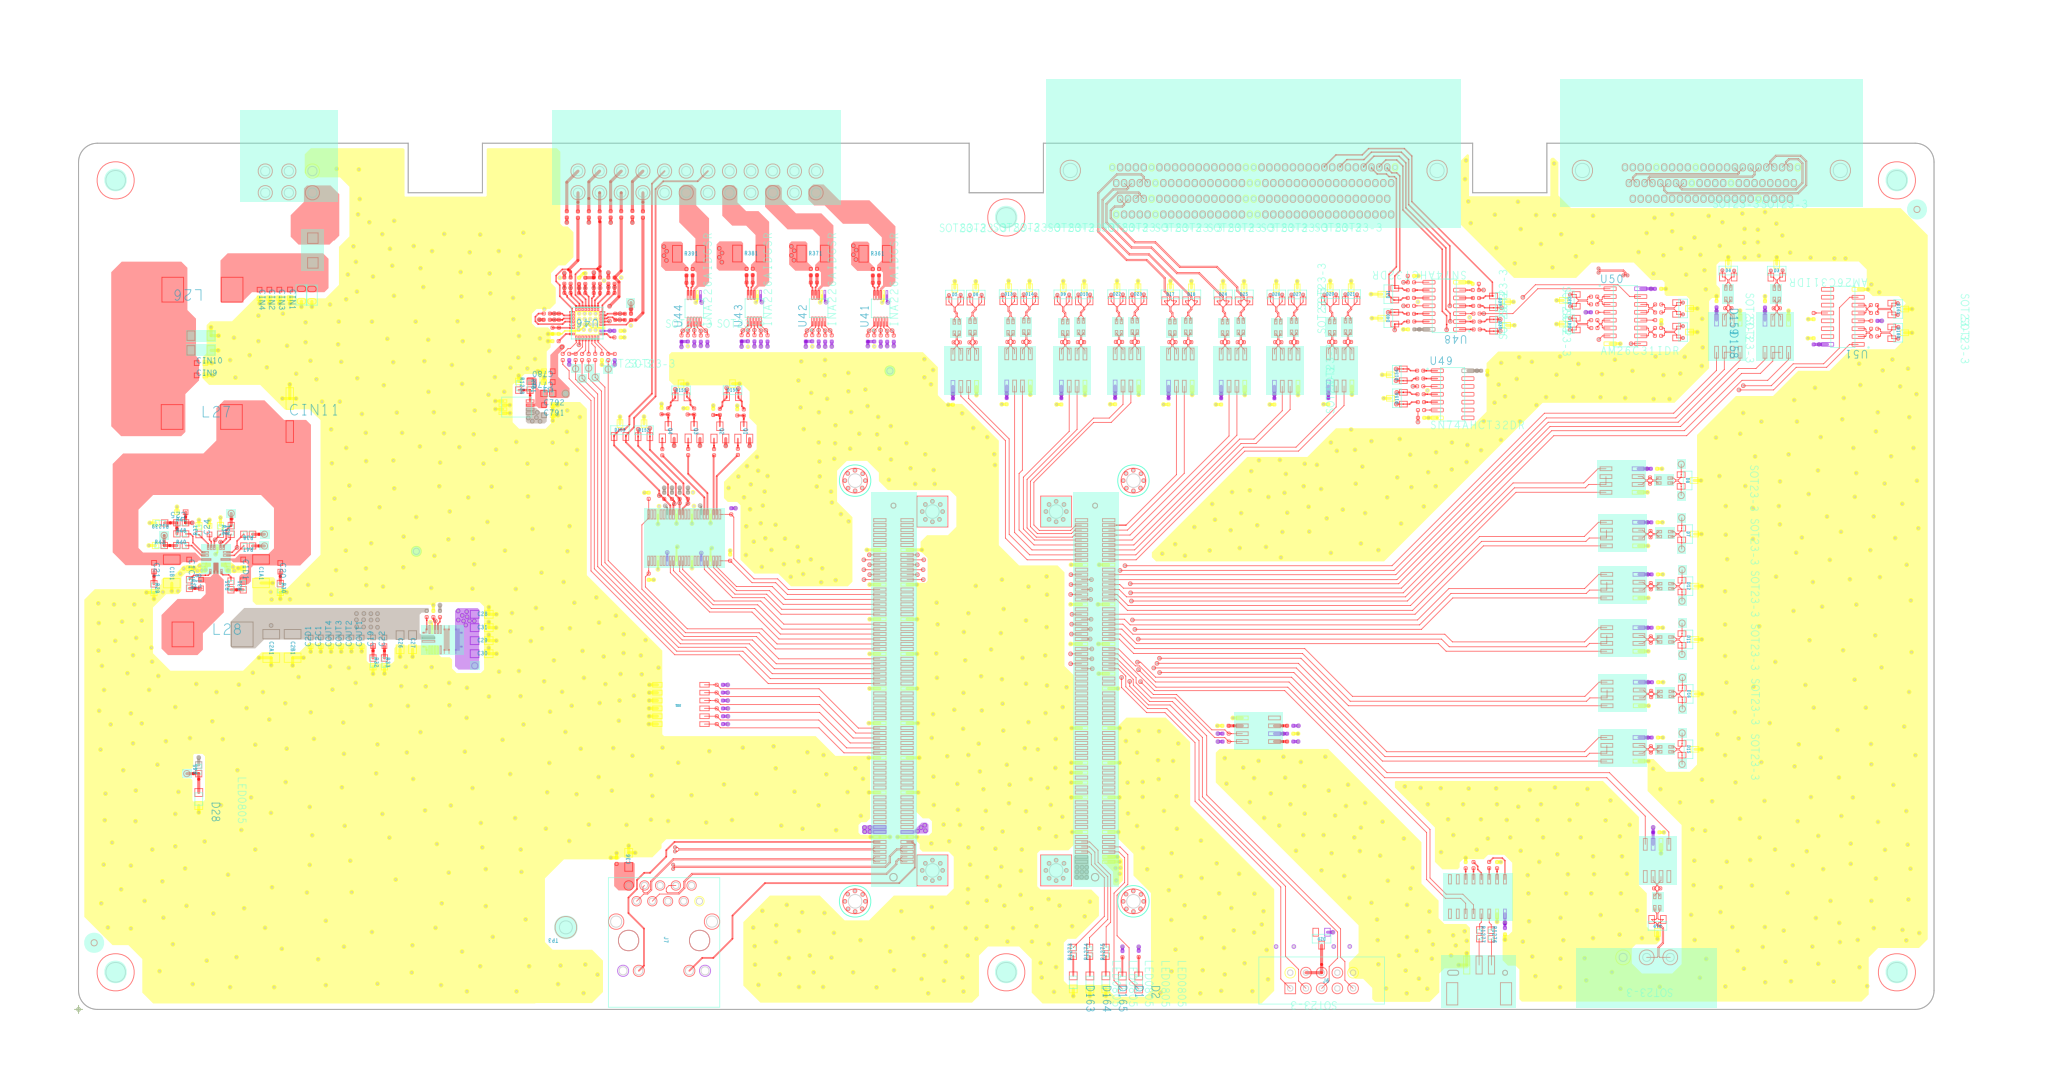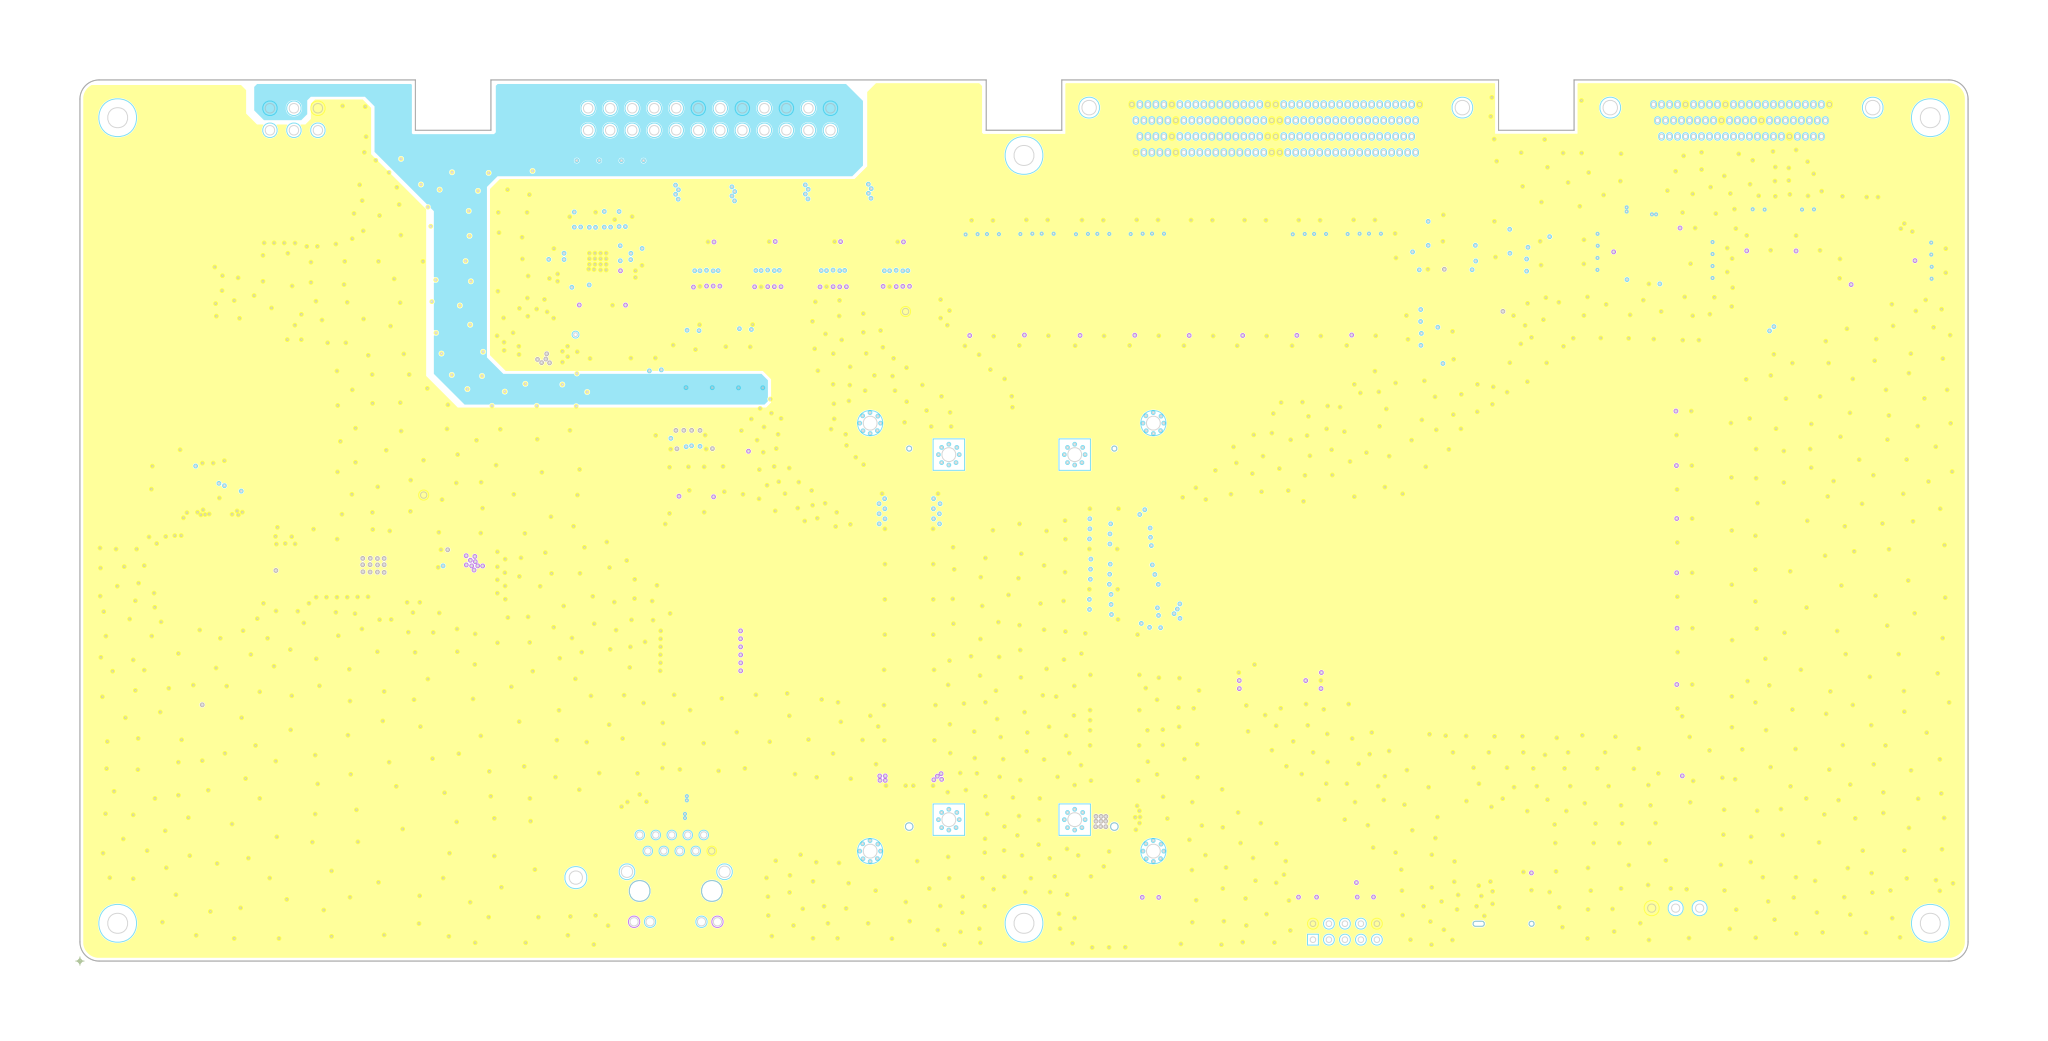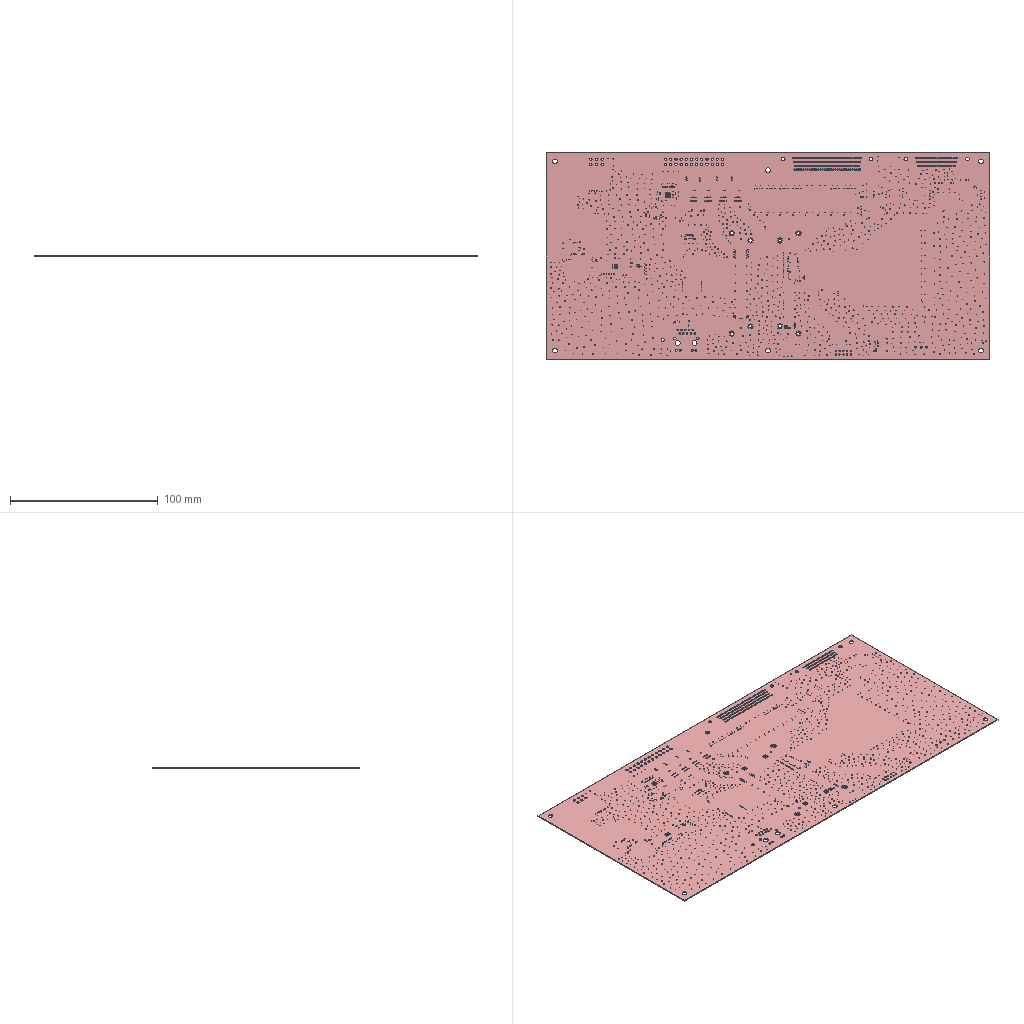Circuit board layout | Cadence Allegro | box 300 x 140 x 0.7 mm
Layer stack:
# Cadence Allegro layer stack of  (unit mm; from the constraint file cross-section; dielectric type: 0 not recorded (Allegro does not mark core vs prepreg), 3 surface material)
index,name,kind,layer,copper_thickness_mm,dielectric_type,dielectric_thickness_mm,dielectric_material,dielectric_constant
0,Top Surface,other,,,,,,
1,TOP,copper,TOP,0.0305,,,,
2,Dielectric1,dielectric,,,0,0.2032,FR-4,4.5
3,GND,copper,GND,0.0305,,,,
4,Dielectric2,dielectric,,,0,0.2032,FR-4,4.5
5,POWER,copper,POWER,0.0305,,,,
6,Dielectric3,dielectric,,,0,0.2032,FR-4,4.5
7,BOTTOM,copper,BOTTOM,0.0305,,,,
8,Bottom Surface,other,,,,,,
# drill layer pairs: low layer,high layer
drill_pair,TOP,BOTTOM
Part placement, first 450 of 481 lines:
REFDES,COMP_VALUE,SYM_NAME,SYM_X,SYM_Y,SYM_ROTATE,SYM_MIRROR
C1A1,CAP/1210,1210,1161.556,2788.237,270.000,NO
C1B1,CAP/1210,1210,593.485,2787.296,270.000,NO
C1C1,CAP/0603,0603C,703.650,2862.517,270.000,NO
C1D1,CAP/0603,0603C,1047.871,2862.911,270.000,NO
C2A1,CAP/1210,1210,1226.556,2312.684,270.000,NO
C2B1,CAP/1210,1210,1362.776,2312.940,270.000,NO
C2C1,CAP/0603,0603C,1542.141,2311.846,90.000,NO
C2D1,CAP/0603,0603C,1477.574,2311.185,90.000,NO
C1,0.1uF/50V/10%/X7R/C0402,0402,10735.047,4486.560,90.000,NO
C2,0.1uF/50V/10%/X7R/C0402,0402,10426.545,4487.348,90.000,NO
C3,0.1uF/50V/10%/X7R/C0402,0402,5565.683,3867.669,270.000,NO
C4,0.1uF/50V/10%/X7R/C0402,0402,10031.322,3099.475,0.000,NO
C5,0.1uF/50V/10%/X7R/C0402,0402,10028.170,3440.285,0.000,NO
C6,0.1uF/50V/10%/X7R/C0402,0402,6255.971,3869.245,270.000,NO
C7,0.1uF/50V/10%/X7R/C0402,0402,10033.292,2428.887,0.000,NO
C8,0.1uF/50V/10%/X7R/C0402,0402,10033.292,2768.121,0.000,NO
C9,0.1uF/50V/10%/X7R/C0402,0402,5908.069,3870.427,270.000,NO
C10,0.1uF/50V/10%/X7R/C0402,0402,10033.686,1729.931,0.000,NO
C11,0.1uF/50V/10%/X7R/C0402,0402,10035.262,2082.167,0.000,NO
C12,0.1uF/50V/10%/X7R/C0402,0402,6938.379,3869.245,270.000,NO
C13,0.1uF/50V/10%/X7R/C0402,0402,10042.870,1126.850,0.000,NO
C14,0.1uF/50V/10%/X7R/C0402,0402,7955.293,3870.427,270.000,NO
C15,0.1uF/50V/10%/X7R/C0402,0402,6598.357,3870.427,270.000,NO
C16,0.1uF/50V/10%/X7R/C0402,0402,7273.279,3868.851,270.000,NO
C17,0.1uF/50V/10%/X7R/C0402,0402,7612.119,3868.851,270.000,NO
C18,CAP/0603,0603C,779.666,2679.579,90.000,NO
C19,CAP/0603,0603C,1874.712,2312.206,90.000,NO
C20,CAP/0603,0603C,1283.974,2840.536,270.000,NO
C21,CAP/0603,0603C,480.432,2841.595,270.000,NO
C22,CAP/0603,0603C,1947.153,2311.572,90.000,NO
C23,CAP/0603,0603C,966.268,3019.048,0.000,YES
C24,CAP/0603,0603C,833.760,3022.493,90.000,NO
C25,CAP/0603,0603C,681.604,3164.030,180.000,NO
C26,22uF/10V/10%/X5R/C0805,0805,2046.721,2336.738,270.000,NO
C27,22uF/10V/10%/X5R/C0805,0805,2126.106,2337.116,270.000,NO
C28,22uF/10V/10%/X5R/C0805,0805,2566.613,2514.273,0.000,NO
C29,22uF/10V/10%/X5R/C0805,0805,2566.125,2346.541,0.000,NO
C30,22uF/10V/10%/X5R/C0805,0805,2566.015,2263.470,0.000,NO
C31,22uF/10V/10%/X5R/C0805,0805,2566.409,2429.265,0.000,NO
C32,39pF/6.3V/5%/NP0/C0402,0402,2258.566,2515.860,270.000,YES
C33,1uF/16V/10%/X5R/C0402,0402,7712.400,1754.535,180.000,NO
C34,0.1uF/50V/10%/X7R/C0402,0402,7712.443,1754.827,0.000,YES
C35,0.1uF/50V/10%/X7R/C0402,0402,7300.619,1804.789,180.000,NO
C36,1uF/50V/10%/X7R/C0805,0805,3501.969,951.575,90.000,NO
C37,0.1uF/50V/10%/X7R/C0402,0402,3424.952,945.752,90.000,NO
C38,0.1uF/50V/10%/X7R/C0402,0402,8482.930,4327.236,180.000,NO
C58,0.1uF/50V/10%/X7R/C0402,0402,5125.368,4545.188,0.000,YES
C59,0.1uF/50V/10%/X7R/C0402,0402,5075.545,4623.152,0.000,NO
C60,0.1uF/50V/10%/X7R/C0402,0402,4730.580,4546.370,0.000,YES
C61,0.1uF/50V/10%/X7R/C0402,0402,4680.757,4624.334,0.000,NO
C62,0.1uF/50V/10%/X7R/C0402,0402,4321.608,4546.764,0.000,YES
C63,0.1uF/50V/10%/X7R/C0402,0402,4271.785,4624.728,0.000,NO
C64,0.1uF/50V/10%/X7R/C0402,0402,3939.034,4545.188,0.000,YES
C65,0.1uF/50V/10%/X7R/C0402,0402,3889.211,4623.152,0.000,NO
C66,0.1uF/50V/10%/X7R/C0402,0402,3936.897,3169.078,180.000,YES
C67,0.1uF/50V/10%/X7R/C0402,0402,3714.884,3167.151,180.000,YES
C68,0.1uF/50V/10%/X7R/C0402,0402,3983.539,2935.806,0.000,YES
C69,0.1uF/50V/10%/X7R/C0402,0402,3767.398,2944.261,0.000,YES
C70,10nF/50V/10%/X7R/C0402,0402,3496.414,4386.724,180.000,YES
C71,0.1uF/50V/10%/X7R/C0402,0402,3416.246,4407.410,90.000,NO
C72,10nF/50V/10%/X7R/C0402,0402,3497.201,4426.307,180.000,YES
C73,0.1uF/50V/10%/X7R/C0402,0402,3188.677,4284.181,270.000,YES
C74,1uF/50V/10%/X7R/C0402,0402,3228.740,4284.122,270.000,YES
C75,0.1uF/50V/10%/X7R/C0402,0402,3057.905,4318.154,270.000,NO
C76,1uF/50V/10%/X7R/C0402,0402,3016.913,4317.992,270.000,NO
C77,10nF/50V/10%/X7R/C0402,0402,3412.091,4636.960,270.000,YES
C78,0.1uF/50V/10%/X7R/C0402,0402,3392.194,4558.369,180.000,NO
C79,10nF/50V/10%/X7R/C0402,0402,3372.509,4637.747,270.000,YES
C80,0.1uF/50V/10%/X7R/C0402,0402,3036.539,4252.260,180.000,NO
C81,0.1uF/50V/10%/X7R/C0402,0402,3430.742,4276.118,0.000,NO
C82,0.1uF/50V/10%/X7R/C0402,0402,3430.262,4318.095,0.000,NO
C83,1uF/50V/10%/X7R/C0402,0402,3332.355,4337.687,270.000,YES
C84,10nF/50V/10%/X7R/C0402,0402,3319.572,4636.960,270.000,YES
C85,0.1uF/50V/10%/X7R/C0402,0402,3299.674,4557.975,180.000,NO
C86,10nF/50V/10%/X7R/C0402,0402,3279.989,4637.748,270.000,YES
C87,10nF/50V/10%/X7R/C0402,0402,3132.170,4637.354,270.000,YES
C88,0.1uF/50V/10%/X7R/C0402,0402,3112.272,4558.762,180.000,NO
C89,10nF/50V/10%/X7R/C0402,0402,3092.193,4637.747,270.000,YES
C92,10nF/50V/10%/X7R/C0402,0402,2981.150,4427.843,0.000,YES
C93,0.1uF/50V/10%/X7R/C0402,0402,3057.772,4407.945,270.000,NO
C94,10nF/50V/10%/X7R/C0402,0402,2980.363,4388.260,0.000,YES
C95,0.1uF/50V/10%/X7R/C0402,0402,3205.579,4557.975,180.000,NO
C96,10nF/50V/10%/X7R/C0402,0402,3225.477,4636.172,270.000,YES
C97,10nF/50V/10%/X7R/C0402,0402,3185.874,4636.172,90.000,NO
C601,0.1uF/50V/10%/X7R/C0402,0402,9079.693,497.732,270.000,NO
C602,0.1uF/50V/10%/X7R/C0402,0402,8978.906,918.744,270.000,NO
C603,0.1uF/50V/10%/X7R/C0402,0402,9029.362,918.118,90.000,NO
C604,0.1uF/50V/10%/X7R/C0402,0402,8829.693,917.854,270.000,NO
C605,0.1uF/50V/10%/X7R/C0402,0402,8879.693,918.000,270.000,NO
C779,10uF/10V/10%/X5R/C0603,0603C,3018.267,3992.411,180.000,NO
C780,0.1uF/50V/10%/X7R/C0603,0603C,3018.267,4060.918,180.000,NO
C791,1uF/25V/10%/X7R/C0603,0603C,2963.148,3780.596,0.000,NO
C792,1uF/25V/10%/X7R/C0603,0603C,2962.944,3845.565,0.000,NO
C793,0.1uF/50V/10%/X7R/C0402,0402,8948.031,4064.173,0.000,NO
C794,0.1uF/50V/10%/X7R/C0402,0402,10054.016,4585.443,0.000,NO
C795,0.1uF/50V/10%/X7R/C0402,0402,11044.795,4251.181,90.000,NO
C796,10nF/50V/10%/X7R/C0402,0402,3728.174,3267.919,270.000,YES
C797,10nF/50V/10%/X7R/C0402,0402,3777.558,3267.589,270.000,YES
C798,10nF/50V/10%/X7R/C0402,0402,3826.614,3267.918,270.000,YES
C799,10nF/50V/10%/X7R/C0402,0402,3879.291,3268.247,270.000,YES
CIN1,CAP/0603,0603C,1345.661,4580.929,270.000,NO
CIN2,CAP/0603,0603C,1214.559,4580.283,270.000,NO
CIN3,CAP/0603,0603C,1277.945,4580.157,270.000,NO
CIN4,CAP/0603,0603C,1152.346,4579.657,270.000,NO
CIN5,CAP/0603,0805C,1485.343,4545.217,270.000,NO
CIN6,CAP/0603,0805C,1418.937,4546.398,270.000,NO
CIN7,CAP/0603,1206,779.079,4193.706,0.000,NO
CIN8,CAP/0603,1206,779.413,4287.245,0.000,NO
CIN9,CAP/0603,0603C,751.999,4034.342,0.000,NO
CIN10,CAP/0603,0603C,752.283,4112.698,0.000,NO
CIN11,CAP/ELECT/DIP/OD5.3P2.0,AP-SMD_BD6_3-L6_6-W6_6-LS7_21,1344.481,3782.142,90.000,NO
COUT1,CAP/0603,0603C,1802.179,2311.008,90.000,NO
COUT2,CAP/0603,0603C,1736.951,2311.402,90.000,NO
COUT3,CAP/0603,0603C,1672.117,2311.007,90.000,NO
COUT4,CAP/0603,0603C,1607.676,2311.006,90.000,NO
D1,LED_GREEN,LED0805,6644.306,171.159,270.000,NO
D2,LED_GREEN,LED0805,6748.087,171.554,270.000,NO
D3,PESD5V0L2BT,SOT23,10809.664,4700.812,0.000,NO
D4,PESD5V0L2BT,SOT23,10501.162,4701.600,0.000,NO
D5,PESD5V0L2BT,SOT23,5577.745,4548.480,0.000,NO
D6,PESD5V0L2BT,SOT23,5711.201,4548.512,0.000,NO
D7,PESD5V0L2BT,SOT23,10245.574,3024.858,270.000,NO
D8,PESD5V0L2BT,SOT23,10242.422,3365.668,270.000,NO
D9,PESD5V0L2BT,SOT23,6268.033,4550.056,0.000,NO
D10,PESD5V0L2BT,SOT23,6401.489,4550.088,0.000,NO
D11,PESD5V0L2BT,SOT23,10247.544,2354.270,270.000,NO
D12,PESD5V0L2BT,SOT23,10247.544,2693.504,270.000,NO
D13,PESD5V0L2BT,SOT23,5920.131,4551.238,0.000,NO
D14,PESD5V0L2BT,SOT23,6053.587,4551.270,0.000,NO
D15,PESD5V0L2BT,SOT23,10247.938,1655.314,270.000,NO
D16,PESD5V0L2BT,SOT23,10249.514,2007.550,270.000,NO
D17,PESD5V0L2BT,SOT23,6950.441,4550.056,0.000,NO
D18,PESD5V0L2BT,SOT23,7083.897,4550.088,0.000,NO
D19,PESD5V0L2BT,SOT23,10050.566,531.402,180.000,NO
D20,PESD5V0L2BT,SOT23,7967.355,4551.238,0.000,NO
D21,PESD5V0L2BT,SOT23,8100.811,4551.270,0.000,NO
D22,PESD5V0L2BT,SOT23,6610.419,4551.238,0.000,NO
D23,PESD5V0L2BT,SOT23,6743.875,4551.270,0.000,NO
D24,PESD5V0L2BT,SOT23,7285.341,4549.662,0.000,NO
D25,PESD5V0L2BT,SOT23,7418.797,4549.694,0.000,NO
D26,PESD5V0L2BT,SOT23,7624.181,4549.662,0.000,NO
D27,PESD5V0L2BT,SOT23,7757.637,4549.694,0.000,NO
D28,LED_GREEN,LED0805,765.200,1338.787,270.000,NO
D29,BAT54C,SOT23,7912.457,450.078,180.000,NO
D30,PESD5V0L2BT,SOT23,9048.678,4353.220,270.000,NO
D31,PESD5V0L2BT,SOT23,8337.260,4551.252,90.000,NO
D32,PESD5V0L2BT,SOT23,9492.519,4511.810,90.000,NO
D39,PESD5V0L2BT,SOT23,9047.890,4502.433,270.000,NO
D40,PESD5V0L2BT,SOT23,8337.260,4398.496,90.000,NO
D41,PESD5V0L2BT,SOT23,9492.519,4361.021,90.000,NO
D150,PESD5V0L2BT,SOT23,4162.815,3940.442,0.000,NO
D151,PESD5V0L2BT,SOT23,3835.260,3939.228,0.000,NO
D152,PESD5V0L2BT,SOT23,3599.433,3685.654,0.000,NO
D153,PESD5V0L2BT,SOT23,3446.504,3686.614,0.000,NO
D154,PESD5V0L2BT,SOT23,8391.339,4038.189,90.000,NO
D155,PESD5V0L2BT,SOT23,8392.126,3888.976,90.000,NO
D158,PESD5V0L2BT,SOT23,10213.779,4310.235,270.000,NO
D159,PESD5V0L2BT,SOT23,10213.780,4460.234,270.000,NO
D160,PESD5V0L2BT,SOT23,11583.070,4305.512,270.000,NO
D161,PESD5V0L2BT,SOT23,11583.465,4456.696,270.000,NO
D162,SS34,DO-214AC,1491.465,4828.969,270.000,NO
D163,LED_GREEN,LED0805,6331.922,172.230,270.000,NO
D164,LED_GREEN,LED0805,6437.434,171.710,270.000,NO
D165,LED_GREEN,LED0805,6539.009,172.371,270.000,NO
E13,Inductor_BEAD,0603R,2990.577,3919.557,0.000,NO
E14,Inductor_BEAD,0603R,2409.882,5042.215,90.000,YES
E15,Inductor_BEAD,0603R,2326.596,5042.215,90.000,YES
E16,Inductor_BEAD,0603R,2241.994,5041.886,90.000,YES
E17,Inductor_BEAD,0603R,2158.050,5042.215,90.000,YES
J1,D2_3,D2_3,5435.335,3168.020,180.000,NO
J2,D2_3,D2_3,6222.736,3168.020,180.000,NO
J3,D2_3,D2_3,6222.736,884.551,180.000,NO
J4,D2_3,D2_3,5435.335,884.551,180.000,NO
J5,BM03B-PASS,JK2EDGRC-381-3_S,10131.890,331.102,0.000,NO
J6,TC2050_IDC_FP1,JTAG-10,7712.992,133.858,0.000,NO
J7,HR911130A,GE_RJ45,3501.181,438.583,270.000,NO
J8,J30JA-144ZKW-J,J30JA-144ZKW-J,7480.315,5338.583,180.000,NO
J9,J30JA-66ZKW-J,J30JA-66ZKW-J,10393.701,5338.583,180.000,NO
J10,BM03B-PASS,BM03B-PASS,8915.248,282.409,0.000,NO
JX1,5177984-6,5177983-6,5187.303,2026.287,90.000,NO
JX2,5177984-6,5177983-6,6470.768,2026.287,90.000,NO
L1,ACM2012H-900-2P-T03,ACM2012,5590.273,4338.796,90.000,NO
L2,ACM2012H-900-2P-T03,ACM2012,10809.991,4553.740,90.000,NO
L3,ACM2012H-900-2P-T03,ACM2012,10501.489,4554.528,90.000,NO
L4,ACM2012H-900-2P-T03,ACM2012,5690.666,4343.268,90.000,NO
L5,ACM2012H-900-2P-T03,ACM2012,10098.502,3024.531,0.000,NO
L6,ACM2012H-900-2P-T03,ACM2012,10095.350,3365.341,0.000,NO
L7,ACM2012H-900-2P-T03,ACM2012,6280.561,4340.372,90.000,NO
L8,ACM2012H-900-2P-T03,ACM2012,6380.954,4344.844,90.000,NO
L9,ACM2012H-900-2P-T03,ACM2012,10100.472,2353.943,0.000,NO
L10,ACM2012H-900-2P-T03,ACM2012,10100.472,2693.177,0.000,NO
L11,ACM2012H-900-2P-T03,ACM2012,5932.659,4341.554,90.000,NO
L12,ACM2012H-900-2P-T03,ACM2012,6033.052,4346.026,90.000,NO
L13,ACM2012H-900-2P-T03,ACM2012,10100.866,1654.987,0.000,NO
L14,ACM2012H-900-2P-T03,ACM2012,10102.442,2007.223,0.000,NO
L15,ACM2012H-900-2P-T03,ACM2012,6962.969,4340.372,90.000,NO
L16,ACM2012H-900-2P-T03,ACM2012,7063.362,4344.844,90.000,NO
L17,ACM2012H-900-2P-T03,ACM2012,7979.883,4341.554,90.000,NO
L18,ACM2012H-900-2P-T03,ACM2012,10049.280,683.035,270.000,NO
L19,ACM2012H-900-2P-T03,ACM2012,8080.276,4346.026,90.000,NO
L20,ACM2012H-900-2P-T03,ACM2012,6622.947,4341.554,90.000,NO
L21,ACM2012H-900-2P-T03,ACM2012,6723.340,4346.026,90.000,NO
L22,ACM2012H-900-2P-T03,ACM2012,7297.869,4339.978,90.000,NO
L23,ACM2012H-900-2P-T03,ACM2012,7636.709,4339.978,90.000,NO
L24,ACM2012H-900-2P-T03,ACM2012,7398.262,4344.450,90.000,NO
L25,ACM2012H-900-2P-T03,ACM2012,7737.102,4344.450,90.000,NO
L26,CKST1004-1uH/M-B,SMD_10X11,788.583,4579.921,180.000,NO
L27,CKST1004-4.7uH/M,SMD_10X11,784.465,3769.807,0.000,NO
L28,CKST1004-4.7uH/M,SMD_10X11,853.146,2386.403,0.000,NO
P1,F83-S-3.81-6pin,F83-S-3_81-6PIN,1338.583,5196.850,180.000,NO
P2,F83-S-3.5-24pin,F83-S-3_5-24PIN,3937.008,5196.850,180.000,NO
Q1,S8050,SOT-23,4234.126,3671.323,270.000,NO
Q2,S8050,SOT-23,4082.157,3671.535,270.000,NO
Q3,S8050,SOT-23,3917.984,3672.535,270.000,NO
Q4,S8050,SOT-23,3753.717,3673.228,270.000,NO
R1,1K/62.5mW/1%/R0402,0402,6645.093,351.474,90.000,NO
R2,1K/62.5mW/1%/R0402,0402,6748.481,353.050,90.000,NO
R3,120R/62.5mW/1%/R0402,0402,5590.253,4244.752,0.000,NO
R4,120R/62.5mW/1%/R0402,0402,10810.057,4461.434,0.000,NO
R5,120R/62.5mW/1%/R0402,0402,10501.555,4462.222,0.000,NO
R6,120R/62.5mW/1%/R0402,0402,5690.748,4244.752,0.000,NO
R7,120R/62.5mW/1%/R0402,0402,10006.196,3024.465,270.000,NO
R8,120R/62.5mW/1%/R0402,0402,10003.044,3365.275,270.000,NO
R9,120R/62.5mW/1%/R0402,0402,6280.541,4246.328,0.000,NO
R10,120R/62.5mW/1%/R0402,0402,6381.036,4246.328,0.000,NO
R11,120R/62.5mW/1%/R0402,0402,10008.166,2353.877,270.000,NO
R12,120R/62.5mW/1%/R0402,0402,10008.166,2693.111,270.000,NO
R13,120R/62.5mW/1%/R0402,0402,5932.639,4247.510,0.000,NO
R14,120R/62.5mW/1%/R0402,0402,6033.134,4247.510,0.000,NO
R15,120R/62.5mW/1%/R0402,0402,10008.560,1654.921,270.000,NO
R16,120R/62.5mW/1%/R0402,0402,10010.136,2007.157,270.000,NO
R17,120R/62.5mW/1%/R0402,0402,6962.949,4246.328,0.000,NO
R18,120R/62.5mW/1%/R0402,0402,7063.444,4246.328,0.000,NO
R19,120R/62.5mW/1%/R0402,0402,7979.863,4247.510,0.000,NO
R20,120R/62.5mW/1%/R0402,0402,10048.657,770.260,180.000,NO
R21,120R/62.5mW/1%/R0402,0402,8080.358,4247.510,0.000,NO
R22,120R/62.5mW/1%/R0402,0402,6622.927,4247.510,0.000,NO
R23,120R/62.5mW/1%/R0402,0402,6723.422,4247.510,0.000,NO
R24,120R/62.5mW/1%/R0402,0402,7297.849,4245.934,0.000,NO
R25,120R/62.5mW/1%/R0402,0402,7636.689,4245.934,0.000,NO
R26,120R/62.5mW/1%/R0402,0402,7398.344,4245.934,0.000,NO
R27,120R/62.5mW/1%/R0402,0402,7737.184,4245.934,0.000,NO
R28,0/62.5mW/1%/R0603,0603R,706.190,2707.005,270.000,NO
R29,10/62.5mW/1%/R0603,0603R,480.124,2680.598,270.000,NO
R30,10/62.5mW/1%/R0603,0603R,1284.286,2682.172,270.000,NO
R31,100K/62.5mW/1%/R0603,0603R,1048.260,2697.690,90.000,NO
R32,10/62.5mW/1%/R0603,0603R,1874.456,2208.513,270.000,NO
R33,10/62.5mW/1%/R0603,0603R,1947.224,2208.513,270.000,NO
R34,100K/62.5mW/1%/R0603,0603R,938.449,3084.355,180.000,YES
R35,10/62.5mW/1%/R0603,0603R,970.162,2697.741,90.000,NO
R36,19.6K/62.5mW/1%/R0603,0603R,903.453,3050.922,270.000,NO
R37,62K/62.5mW/1%/R0603,0603R,766.225,3049.568,90.000,NO
R38,10/62.5mW/1%/R0603,0603R,1080.012,3023.497,180.000,NO
R39,100K/62.5mW/1%/R0603,0603R,931.686,2933.740,180.000,YES
R40,10/62.5mW/1%/R0603,0603R,653.304,2951.670,0.000,NO
R41,10/62.5mW/1%/R0603,0603R,653.430,3096.551,0.000,NO
R43,51K/62.5mW/1%/R0603,0603R,517.852,2952.065,0.000,NO
R45,10K/62.5mW/1%/R0603,0603R,765.055,1527.969,90.000,NO
R47,10/62.5mW/1%/R0603,0603R,1079.863,2949.355,180.000,NO
R48,10/62.5mW/1%/R0603,0603R,653.804,3025.993,0.000,NO
R51,10/62.5mW/1%/R0603,0603R,971.808,3050.840,90.000,NO
R52,499K/62.5mW/1%/R0402,0402,2300.535,2515.711,270.000,NO
R53,100k/62.5mW/1%/R0402,0402,2216.086,2516.065,90.000,NO
R54,20K/62.5mW/1%/R0402,0402,2300.550,2515.711,90.000,YES
R55,4.42K/62.5mW/1%/R0402,0402,2258.542,2515.931,270.000,NO
R61,4.7K/62.5mW/1%/R0402,0402,7712.576,1804.891,180.000,NO
R62,4.7K/62.5mW/1%/R0402,0402,7712.619,1704.496,180.000,NO
R63,4.7K/62.5mW/1%/R0402,0402,7302.166,1704.119,0.000,NO
R64,4.7K/62.5mW/1%/R0402,0402,7301.422,1754.906,0.000,NO
R65,4.7K/62.5mW/1%/R0402,0402,7651.480,380.210,90.000,YES
R66,4.7K/62.5mW/1%/R0402,0402,7766.922,380.210,90.000,YES
R67,4.7K/62.5mW/1%/R0402,0402,7963.528,380.604,90.000,YES
R68,4.7K/62.5mW/1%/R0402,0402,8063.210,380.998,90.000,YES
R69,10K/62.5mW/1%/R0402,0402,4081.841,2065.463,180.000,NO
R70,10K/62.5mW/1%/R0402,0402,4081.448,2016.069,180.000,NO
R71,10K/62.5mW/1%/R0402,0402,4081.841,1965.493,180.000,NO
R72,10K/62.5mW/1%/R0402,0402,4082.235,1915.313,180.000,NO
R73,10K/62.5mW/1%/R0402,0402,4082.597,1865.431,180.000,NO
R74,10K/62.5mW/1%/R0402,0402,4082.329,1815.675,180.000,NO
R75,0R/62.5mW/1%/R0402,0402,3304.330,539.259,270.000,YES
R76,10/62.5mW/1%/R0402,0402,8899.859,4326.842,180.000,NO
R78,10/62.5mW/1%/R0402,0402,8899.465,4376.842,180.000,NO
R85,10/62.5mW/1%/R0402,0402,8897.103,4476.842,180.000,NO
R88,1k/62.5mW/1%/R0402,0402,8898.678,4427.630,0.000,NO
R89,1k/62.5mW/1%/R0402,0402,8894.347,4577.630,0.000,NO
R91,1k/62.5mW/1%/R0402,0402,8481.355,4626.842,180.000,NO
R94,1k/62.5mW/1%/R0402,0402,8481.749,4476.842,180.000,NO
R97,10/62.5mW/1%/R0402,0402,8895.134,4526.842,180.000,NO
R100,22/62.5mW/1%/R0402,0402,8482.536,4377.236,180.000,NO
R103,22/62.5mW/1%/R0402,0402,8481.749,4426.055,180.000,NO
R109,22/62.5mW/1%/R0402,0402,8480.961,4527.236,180.000,NO
R112,22/62.5mW/1%/R0402,0402,8480.567,4576.842,180.000,NO
R356,10k/62.5mW/1%/R0402,0402,5064.908,4269.718,90.000,NO
R357,10k/62.5mW/1%/R0402,0402,5024.176,4269.324,90.000,NO
R358,10k/62.5mW/1%/R0402,0402,5064.940,4269.615,90.000,YES
R359,10k/62.5mW/1%/R0402,0402,5024.208,4269.222,90.000,YES
R360,4.7R/62.5mW/1%/R0402,0402,5056.057,4690.656,90.000,NO
R361,20m/0.5W/0.01%/R1210,1210,5071.789,4808.309,0.000,NO
R362,4.7R/62.5mW/1%/R0402,0402,5095.246,4691.443,90.000,NO
R363,10k/62.5mW/1%/R0402,0402,5106.168,4269.222,270.000,NO
R364,10k/62.5mW/1%/R0402,0402,5189.420,4268.434,270.000,NO
R365,10k/62.5mW/1%/R0402,0402,5147.404,4268.529,270.000,NO
R366,10k/62.5mW/1%/R0402,0402,4670.120,4270.900,90.000,NO
R367,10k/62.5mW/1%/R0402,0402,4629.388,4270.506,90.000,NO
R368,10k/62.5mW/1%/R0402,0402,4670.152,4270.797,90.000,YES
R369,10k/62.5mW/1%/R0402,0402,4629.420,4270.404,90.000,YES
R370,4.7R/62.5mW/1%/R0402,0402,4661.269,4691.838,90.000,NO
R371,20m/0.5W/0.01%/R1210,1210,4677.001,4809.491,0.000,NO
R372,4.7R/62.5mW/1%/R0402,0402,4700.458,4692.625,90.000,NO
R373,10k/62.5mW/1%/R0402,0402,4711.380,4270.404,270.000,NO
R374,10k/62.5mW/1%/R0402,0402,4794.632,4269.616,270.000,NO
R375,10k/62.5mW/1%/R0402,0402,4752.616,4269.711,270.000,NO
R376,10k/62.5mW/1%/R0402,0402,4261.148,4271.294,90.000,NO
R377,10k/62.5mW/1%/R0402,0402,4220.416,4270.900,90.000,NO
R378,10k/62.5mW/1%/R0402,0402,4261.180,4271.191,90.000,YES
R379,10k/62.5mW/1%/R0402,0402,4220.448,4270.798,90.000,YES
R380,4.7R/62.5mW/1%/R0402,0402,4252.297,4692.232,90.000,NO
R381,20m/0.5W/0.01%/R1210,1210,4268.029,4809.885,0.000,NO
R382,4.7R/62.5mW/1%/R0402,0402,4291.486,4693.019,90.000,NO
R383,10k/62.5mW/1%/R0402,0402,4302.408,4270.798,270.000,NO
R384,10k/62.5mW/1%/R0402,0402,4385.660,4270.010,270.000,NO
R385,10k/62.5mW/1%/R0402,0402,4343.644,4270.105,270.000,NO
R386,10k/62.5mW/1%/R0402,0402,3878.574,4269.718,90.000,NO
R387,10k/62.5mW/1%/R0402,0402,3837.842,4269.324,90.000,NO
R388,10k/62.5mW/1%/R0402,0402,3878.606,4269.615,90.000,YES
R389,10k/62.5mW/1%/R0402,0402,3837.874,4269.222,90.000,YES
R390,4.7R/62.5mW/1%/R0402,0402,3869.723,4690.656,90.000,NO
R391,20m/0.5W/0.01%/R1210,1210,3885.455,4808.309,0.000,NO
R392,4.7R/62.5mW/1%/R0402,0402,3908.912,4691.443,90.000,NO
R393,10k/62.5mW/1%/R0402,0402,3919.834,4269.222,270.000,NO
R394,10k/62.5mW/1%/R0402,0402,4003.086,4268.434,270.000,NO
R395,10k/62.5mW/1%/R0402,0402,3961.070,4268.529,270.000,NO
R396,22/62.5mW/0.1%/R0402,0402,4234.741,3798.240,270.000,NO
R397,22/62.5mW/0.1%/R0402,0402,4082.379,3802.324,270.000,NO
R398,22/62.5mW/0.1%/R0402,0402,3918.599,3804.435,270.000,NO
R399,22/62.5mW/0.1%/R0402,0402,3753.639,3805.766,270.000,NO
R400,2.49K/62.5mW/1%/R0402,0402,3879.054,3268.277,90.000,NO
R401,2.49K/62.5mW/1%/R0402,0402,3826.500,3267.883,90.000,NO
R402,2.49K/62.5mW/1%/R0402,0402,3777.493,3267.883,90.000,NO
R403,1k/62.5mW/0.1%/R0402,0402,4197.007,3547.854,270.000,NO
R404,1k/62.5mW/0.1%/R0402,0402,4045.220,3545.886,270.000,NO
R405,1k/62.5mW/0.1%/R0402,0402,3880.440,3546.674,270.000,NO
R406,1k/62.5mW/0.1%/R0402,0402,3715.661,3545.492,270.000,NO
R407,2.49K/62.5mW/1%/R0402,0402,3728.092,3267.883,90.000,NO
R408,10K/62.5mW/1%/R0402,0402,4147.703,2874.331,270.000,NO
R409,10K/62.5mW/1%/R0402,0402,4154.633,3169.550,270.000,NO
R410,10K/62.5mW/1%/R0402,0402,3629.291,2753.587,90.000,NO
R411,10K/62.5mW/1%/R0402,0402,3629.350,3268.445,270.000,NO
R412,0/62.5mW/1%/R0402,0402,3592.579,5058.248,270.000,NO
R413,1K/62.5mW/1%/R0402,0402,3525.497,5060.718,90.000,NO
R414,0/62.5mW/1%/R0402,0402,3454.177,5059.035,270.000,NO
R415,1K/62.5mW/1%/R0402,0402,3387.310,5058.996,90.000,NO
R416,0/62.5mW/1%/R0402,0402,3317.051,5058.094,270.000,NO
R417,1K/62.5mW/1%/R0402,0402,3248.281,5058.858,90.000,NO
R418,0/62.5mW/1%/R0402,0402,3178.767,5057.460,270.000,NO
R419,1K/62.5mW/1%/R0402,0402,3107.939,5058.858,90.000,NO
R420,1K/62.5mW/1%/R0402,0402,3496.524,4386.740,0.000,NO
R421,1K/62.5mW/1%/R0402,0402,3496.918,4426.291,0.000,NO
R422,1K/62.5mW/1%/R0402,0402,3412.075,4637.070,90.000,NO
R423,1K/62.5mW/1%/R0402,0402,3372.524,4637.464,90.000,NO
R424,10k/62.5mW/1%/R0402,0402,3412.995,4151.281,90.000,NO
R425,10k/62.5mW/1%/R0402,0402,3123.460,4151.675,90.000,NO
R426,1K/62.5mW/1%/R0402,0402,3319.556,4637.071,90.000,NO
R427,22/62.5mW/1%/R0402,0402,3164.142,4151.789,270.000,NO
R428,1K/62.5mW/1%/R0402,0402,3280.005,4637.464,90.000,NO
R429,22/62.5mW/1%/R0402,0402,3371.803,4151.395,270.000,NO
R431,10k/62.5mW/1%/R0402,0402,3331.496,4151.864,270.000,NO
R432,22/62.5mW/1%/R0402,0402,3082.188,4151.789,270.000,NO
R433,22/62.5mW/1%/R0402,0402,3247.362,4151.002,270.000,NO
R434,22/62.5mW/1%/R0402,0402,3205.024,4151.395,270.000,NO
R435,1K/62.5mW/1%/R0402,0402,3132.154,4637.464,90.000,NO
R436,22/62.5mW/1%/R0402,0402,3288.669,4151.789,270.000,NO
R437,1K/62.5mW/1%/R0402,0402,3092.209,4637.464,90.000,NO
R438,1K/62.5mW/1%/R0402,0402,2981.040,4427.827,180.000,NO
R439,1K/62.5mW/1%/R0402,0402,2980.646,4388.276,180.000,NO
R440,1K/62.5mW/1%/R0402,0402,3225.461,4636.283,90.000,NO
R441,1K/62.5mW/1%/R0402,0402,3205.978,4752.822,0.000,YES
R442,1K/62.5mW/1%/R0402,0402,3185.858,4635.888,270.000,YES
R443,1K/62.5mW/1%/R0402,0402,3205.978,4707.906,180.000,YES
R781,20K/62.5mW/1%/R0603,0603R,2874.140,3968.352,270.000,NO
R1238,6.34k/62.5mW/1%/R0603,0603R,2801.699,3968.505,270.000,NO
R1239,0/62.5mW/1%/R0603,0603R,520.391,3095.865,180.000,NO
R1244,10/62.5mW/1%/R0402,0402,8540.157,4064.567,0.000,NO
R1245,10/62.5mW/1%/R0402,0402,8540.551,4014.567,0.000,NO
R1246,10/62.5mW/1%/R0402,0402,8544.882,3864.567,0.000,NO
R1247,10/62.5mW/1%/R0402,0402,8542.913,3914.567,0.000,NO
R1248,1k/62.5mW/1%/R0402,0402,8540.157,3964.961,180.000,NO
R1250,1k/62.5mW/1%/R0402,0402,8545.669,3813.780,180.000,NO
R1251,2K/62.5mW/1%/R0402,0402,8482.142,4476.449,0.000,YES
R1252,2K/62.5mW/1%/R0402,0402,8480.961,4667.618,180.000,NO
R1253,2K/62.5mW/1%/R0402,0402,8893.952,4617.148,0.000,NO
R1254,2K/62.5mW/1%/R0402,0402,8898.678,4427.630,180.000,YES
R1255,2K/62.5mW/1%/R0402,0402,8540.157,3964.961,0.000,YES
R1256,2K/62.5mW/1%/R0402,0402,8545.669,3764.567,180.000,NO
R1257,10K/62.5mW/1%/R0402,0402,9646.457,4436.220,0.000,NO
R1258,22/62.5mW/1%/R0402,0402,10055.512,4386.220,0.000,NO
R1259,0/62.5mW/1%/R0402,0402,9648.031,4385.827,0.000,NO
R1260,0/62.5mW/1%/R0402,0402,9647.244,4486.614,0.000,NO
R1261,0/62.5mW/1%/R0402,0402,9647.244,4535.433,0.000,NO
R1262,0/62.5mW/1%/R0402,0402,9648.819,4335.827,0.000,NO
R1263,0/62.5mW/1%/R0402,0402,10055.118,4435.039,180.000,NO
R1264,0/62.5mW/1%/R0402,0402,10054.331,4336.220,180.000,NO
R1265,0/62.5mW/1%/R0402,0402,10053.937,4286.220,180.000,NO
R1266,0/62.5mW/1%/R0402,0402,10055.118,4485.827,180.000,NO
R1267,10K/62.5mW/1%/R0402,0402,11430.709,4381.496,180.000,NO
R1268,22/62.5mW/1%/R0402,0402,11044.882,4411.811,270.000,NO
R1269,0/62.5mW/1%/R0402,0402,11429.134,4431.890,180.000,NO
R1270,0/62.5mW/1%/R0402,0402,11429.921,4331.102,180.000,NO
R1271,0/62.5mW/1%/R0402,0402,11429.921,4282.283,180.000,NO
R1272,0/62.5mW/1%/R0402,0402,11428.346,4481.890,180.000,NO
R1273,10K/62.5mW/1%/R0603,0603R,6332.461,366.281,90.000,NO
R1274,10K/62.5mW/1%/R0603,0603R,6436.005,366.801,90.000,NO
R1275,10K/62.5mW/1%/R0603,0603R,6541.123,366.533,90.000,NO
R1276,10/62.5mW/1%/R0603,0603R,8991.858,476.476,270.000,NO
R1277,10/62.5mW/1%/R0603,0603R,8918.630,477.925,270.000,NO
R1278,10k/62.5mW/0.1%/R0402,0402,4193.052,3798.954,270.000,NO
R1279,10k/62.5mW/0.1%/R0402,0402,4040.287,3802.246,270.000,NO
R1280,10k/62.5mW/0.1%/R0402,0402,3876.987,3805.538,270.000,NO
R1281,10k/62.5mW/0.1%/R0402,0402,3711.053,3806.855,270.000,NO
SW1,SW DIP-6,W-SMD_12P-L9_3-W5_4-P1_27-LS2,3834.648,1940.659,270.000,NO
TP1,TEST POINT A,TEST_12MM,688.977,1500.393,0.000,NO
TP2,TEST POINT A,TEST_12MM,2521.956,2186.801,0.000,NO
TP3,TEST POINT A,HOLE2-3_5,3102.118,522.159,180.000,NO
TP4,TEST POINT A,TEST_12MM,3371.654,4074.407,180.000,NO
TP5,TEST POINT A,TEST_12MM,3163.972,4076.442,180.000,NO
TP6,TEST POINT A,TEST_12MM,3247.244,4080.314,180.000,NO
TP7,TEST POINT A,TEST_12MM,3205.079,4015.486,180.000,NO
TP8,TEST POINT A,TEST_12MM,3288.189,4022.046,180.000,NO
TP9,TEST POINT A,TEST_12MM,3516.560,4498.112,270.000,NO
TP70,CVDD,D0_6,3100.245,3918.617,180.000,NO
TP71,TEST POINT A,TEST_12MM,544.875,3016.325,0.000,NO
TP72,TEST POINT A,TEST_12MM,1183.547,2949.155,180.000,NO
TP73,TEST POINT A,TEST_12MM,1183.511,3023.556,0.000,NO
TP74,TEST POINT A,TEST_12MM,971.812,3156.328,0.000,NO
TP75,TEST POINT A,TEST_12MM,10205.157,3128.753,270.000,NO
TP76,TEST POINT A,TEST_12MM,10204.764,2929.311,270.000,NO
TP77,TEST POINT A,TEST_12MM,10202.005,3469.563,270.000,NO
TP78,TEST POINT A,TEST_12MM,10201.612,3270.121,270.000,NO
TP79,TEST POINT A,TEST_12MM,10207.127,2797.399,270.000,NO
TP80,TEST POINT A,TEST_12MM,10206.734,2597.957,270.000,NO
TP81,TEST POINT A,TEST_12MM,10209.097,2111.445,270.000,NO
TP82,TEST POINT A,TEST_12MM,10208.704,1912.003,270.000,NO
TP83,TEST POINT A,TEST_12MM,10207.521,1759.209,270.000,NO
TP84,TEST POINT A,TEST_12MM,10207.128,1559.767,270.000,NO
TP85,TEST POINT A,TEST_12MM,10207.127,2458.165,270.000,NO
TP86,TEST POINT A,TEST_12MM,10206.734,2258.723,270.000,NO
TP87,TEST POINT A,TEST_1MM,5164.706,4063.270,0.000,NO
TP88,TEST POINT A,TEST_1MM,2150.231,2914.905,0.000,NO
U1,MAX3485ESA+T,SO8,10809.848,4283.406,0.000,NO
Pad and via stacks:
# Allegro (Cadence) via spans and padstacks; design units: ("mils" 3 1000)
# via spans: padstack,start_layer,end_layer,net_example,count
VIA12X20,ETCH/TOP,ETCH/BOTTOM,ETH_MD3_P,48
VIA12_24,ETCH/TOP,ETCH/BOTTOM,AGND,1598
# Allegro padstack definitions: name,start_layer,end_layer,drill,plating,holeType,type
2020B,"ETCH/TOP","ETCH/TOP",0.0,"PLATED","none","smd"
SMD_R551X500P0S40,"ETCH/TOP","ETCH/TOP",0.0,"PLATED","none","smd"
PSM_065X081R,"ETCH/TOP","ETCH/TOP",0.0,"PLATED","none","smd"
SMD50_50,"ETCH/TOP","ETCH/TOP",0.0,"PLATED","none","smd"
SMD200X50,"ETCH/TOP","ETCH/TOP",0.0,"PLATED","none","smd"
R75X85,"ETCH/TOP","ETCH/TOP",0.0,"NON_PLATED","none","smd"
RE55X40,"ETCH/TOP","ETCH/TOP",0.0,"NON_PLATED","none","smd"
SMD_R591X1063P0S40,"ETCH/TOP","ETCH/TOP",0.0,"PLATED","none","smd"
Y10,"ETCH/TOP","ETCH/TOP",0.0,"NON_PLATED","none","smd"
R61X15,"ETCH/TOP","ETCH/TOP",0.0,"NON_PLATED","none","smd"
SMD_S50P0S40,"ETCH/TOP","ETCH/TOP",0.0,"PLATED","none","smd"
SMD_R510X80P0S0,"ETCH/TOP","ETCH/TOP",0.0,"PLATED","none","smd"
SMD_R810X100P0S0,"ETCH/TOP","ETCH/TOP",0.0,"PLATED","none","smd"
S_R197T60D2M197_60P197_60,"ETCH/TOP","ETCH/TOP",0.0,"PLATED","none","smd"
S_R147T28D2M147_28P147_28,"ETCH/TOP","ETCH/TOP",0.0,"PLATED","none","smd"
R150_30_K,"ETCH/TOP","ETCH/TOP",0.0,"NON_PLATED","none","smd"
RX148Y148D0T,"ETCH/TOP","ETCH/TOP",0.0,"PLATED","none","smd"
RX10Y32D0T,"ETCH/TOP","ETCH/TOP",0.0,"PLATED","none","smd"
SMD36_50,"ETCH/TOP","ETCH/TOP",0.0,"PLATED","none","smd"
PSM_091S_PM,"ETCH/TOP","ETCH/TOP",0.0,"NON_PLATED","none","smd"
R105_100,"ETCH/TOP","ETCH/TOP",0.0,"PLATED","none","smd"
BGA10_SMD0X619,"ETCH/TOP","ETCH/TOP",0.0,"NON_PLATED","none","smd"
O0R9X1R4,"ETCH/TOP","ETCH/TOP",0.0,"NON_PLATED","none","smd"
R127X152,"ETCH/TOP","ETCH/TOP",0.0,"NON_PLATED","none","smd"
SMD_R1378X472P0S20,"ETCH/TOP","ETCH/TOP",0.0,"PLATED","none","smd"
SMD_R600X300P0S20,"ETCH/TOP","ETCH/TOP",0.0,"PLATED","none","smd"
SMD_R1378X1575P0S20,"ETCH/TOP","ETCH/TOP",0.0,"PLATED","none","smd"
RX43Y10D0T,"ETCH/TOP","ETCH/TOP",0.0,"PLATED","none","smd"
RX59Y10D0T,"ETCH/TOP","ETCH/TOP",0.0,"PLATED","none","smd"
RX5Y5D0T,"ETCH/TOP","ETCH/TOP",0.0,"PLATED","none","smd"
RX28Y10D0T,"ETCH/TOP","ETCH/TOP",0.0,"PLATED","none","smd"
SMD_S300P0S10,"ETCH/TOP","ETCH/TOP",0.0,"PLATED","none","smd"
Y3_MARK,"ETCH/TOP","ETCH/TOP",0.0,"PLATED","none","smd"
F45,"ETCH/TOP","ETCH/TOP",0.0,"PLATED","none","smd"
R91X127,"ETCH/TOP","ETCH/TOP",0.0,"NON_PLATED","none","smd"
S91,"ETCH/TOP","ETCH/TOP",0.0,"NON_PLATED","none","smd"
R127X120,"ETCH/TOP","ETCH/TOP",0.0,"NON_PLATED","none","smd"
R40X36,"ETCH/TOP","ETCH/TOP",0.0,"PLATED","none","smd"
R127X121,"ETCH/TOP","ETCH/TOP",0.0,"PLATED","none","smd"
R88X76,"ETCH/TOP","ETCH/TOP",0.0,"PLATED","none","smd"
R60X20,"ETCH/TOP","ETCH/TOP",0.0,"PLATED","none","smd"
R120X70,"ETCH/TOP","ETCH/TOP",0.0,"PLATED","none","smd"
R50X32,"ETCH/TOP","ETCH/TOP",0.0,"PLATED","none","smd"
S437,"ETCH/TOP","ETCH/TOP",0.0,"PLATED","none","smd"
Y4,"ETCH/TOP","ETCH/TOP",0.0,"PLATED","none","smd"
SMD0_45R,"ETCH/TOP","ETCH/TOP",0.0,"PLATED","none","smd"
R85X65,"ETCH/TOP","ETCH/TOP",0.0,"PLATED","none","smd"
Y50,"ETCH/TOP","ETCH/TOP",0.0,"PLATED","none","smd"
RE43_31X19_68,"ETCH/TOP","ETCH/TOP",0.0,"PLATED","none","smd"
RE134X170,"ETCH/TOP","ETCH/TOP",0.0,"PLATED","none","smd"
SMD_R98X276P0S30,"ETCH/TOP","ETCH/TOP",0.0,"PLATED","none","smd"
SMD_R98X433P0S30,"ETCH/TOP","ETCH/TOP",0.0,"PLATED","none","smd"
SMD_R98X276P0S10,"ETCH/TOP","ETCH/TOP",0.0,"PLATED","none","smd"
SMD_R98X433P0S10,"ETCH/TOP","ETCH/TOP",0.0,"PLATED","none","smd"
SMD_R236X669P0S40,"ETCH/TOP","ETCH/TOP",0.0,"PLATED","none","smd"
SMD_R236X669P0S30,"ETCH/TOP","ETCH/TOP",0.0,"PLATED","none","smd"
SMD_R98X433S30,"ETCH/TOP","ETCH/TOP",0.0,"PLATED","none","smd"
C12_6,"ETCH/TOP","ETCH/TOP",0.0,"PLATED","none","smd"
R80X25,"ETCH/TOP","ETCH/TOP",0.0,"PLATED","none","smd"
SMD10_61,"ETCH/TOP","ETCH/TOP",0.0,"PLATED","none","smd"
R29_92X50,"ETCH/TOP","ETCH/TOP",0.0,"PLATED","none","smd"
S_R197T60D5M197_60P197_60,"ETCH/TOP","ETCH/TOP",0.0,"PLATED","none","smd"
R36X18,"ETCH/TOP","ETCH/TOP",0.0,"PLATED","none","smd"
R29X10,"ETCH/TOP","ETCH/TOP",0.0,"PLATED","none","smd"
R45X150,"ETCH/TOP","ETCH/TOP",0.0,"NON_PLATED","none","smd"
S17,"ETCH/TOP","ETCH/TOP",0.0,"NON_PLATED","none","smd"
Y24,"ETCH/TOP","ETCH/BOTTOM",51.181,"PLATED","circle_drill","through"
C68_11D35,"ETCH/TOP","ETCH/BOTTOM",35.039,"PLATED","circle_drill","through"
SQ68_11D35,"ETCH/TOP","ETCH/BOTTOM",35.039,"PLATED","circle_drill","through"
C130D130N,"ETCH/TOP","ETCH/BOTTOM",129.921,"NON_PLATED","circle_drill","through"
C98D70_87,"ETCH/TOP","ETCH/BOTTOM",70.87,"PLATED","circle_drill","through"
C70_87D51_18,"ETCH/TOP","ETCH/BOTTOM",51.181,"PLATED","circle_drill","through"
C60D40,"ETCH/TOP","ETCH/BOTTOM",40.0,"PLATED","circle_drill","through"
Y0_80,"ETCH/TOP","ETCH/BOTTOM",31.496,"NON_PLATED","circle_drill","through"
Y0_120,"ETCH/TOP","ETCH/BOTTOM",47.244,"NON_PLATED","circle_drill","through"
Y60,"ETCH/TOP","ETCH/BOTTOM",123.622,"PLATED","circle_drill","through"
Y0_0_6,"ETCH/TOP","ETCH/BOTTOM",23.622,"PLATED","circle_drill","through"
Y1000,"ETCH/TOP","ETCH/BOTTOM",39.37,"PLATED","circle_drill","through"
Y3000,"ETCH/TOP","ETCH/BOTTOM",78.74,"PLATED","circle_drill","through"
VIA24D12,"ETCH/TOP","ETCH/BOTTOM",12.0,"PLATED","circle_drill","through"
Y4_6,"ETCH/TOP","ETCH/BOTTOM",86.614,"PLATED","circle_drill","through"
F152,"ETCH/TOP","ETCH/BOTTOM",40.0,"PLATED","circle_drill","through"
F15,"ETCH/TOP","ETCH/BOTTOM",40.0,"PLATED","circle_drill","through"
Y150_1,"ETCH/TOP","ETCH/BOTTOM",59.055,"PLATED","circle_drill","through"
Y70_120_1,"ETCH/TOP","ETCH/BOTTOM",27.559,"PLATED","circle_drill","through"
Y230_1,"ETCH/TOP","ETCH/BOTTOM",90.551,"PLATED","circle_drill","through"
D3,"ETCH/TOP","ETCH/BOTTOM",118.11,"NON_PLATED","circle_drill","through"
Y328,"ETCH/TOP","ETCH/BOTTOM",129.134,"NON_PLATED","circle_drill","through"
Y300_1,"ETCH/TOP","ETCH/BOTTOM",125.0,"NON_PLATED","circle_drill","through"
Y4_5,"ETCH/TOP","ETCH/BOTTOM",86.614,"PLATED","circle_drill","through"
VIA_D10C020,"ETCH/TOP","ETCH/BOTTOM",10.0,"PLATED","circle_drill","through"
EX63Y63D43P,"ETCH/TOP","ETCH/BOTTOM",43.0,"PLATED","circle_drill","through"
EX83Y83D63P,"ETCH/TOP","ETCH/BOTTOM",63.0,"PLATED","circle_drill","through"
T18X9,"ETCH/TOP","ETCH/BOTTOM",31.496,"NON_PLATED","oval slot","through"
Y8,"ETCH/TOP","ETCH/BOTTOM",31.496,"NON_PLATED","circle_drill","through"
VIA12_24,"ETCH/TOP","ETCH/BOTTOM",11.81,"PLATED","circle_drill","through"
VIA12X20,"ETCH/TOP","ETCH/BOTTOM",12.0,"PLATED","circle_drill","through"
HOLE2-3_5,"ETCH/TOP","ETCH/BOTTOM",82.68,"PLATED","circle_drill","through"
PAD18,"ETCH/TOP","ETCH/TOP",0.0,"NON_PLATED","none","smd"
Design rules, without the lines most boards share, first 9 of 61 lines:
# Cadence Allegro design rules of  (from the Constraint Manager export constraints.dcfx, design unit mil; typed fields in mm)
# columns: name | kind | enabled | priority | scope1 | scope2 | descriptor | typed fields (field=value)
# Allegro precedence (priority 1 wins): 1 Region class-to-class, 2 Region class, 3 Region, 4 class-to-class, 5 DiffPair/Bus/NetGroup override, 6 NetClass, 7 constraint set (CSet) default
# per-layer values are written LAYER=value in the descriptor and LAYER:mm in the typed field; a maximum of 0 means no limit set
# --- net classes (and buses / net groups) ---
# (no net classes defined: every net uses the default constraint sets)
# --- track widths, neck and differential-pair gap (physical constraint sets) ---
DEFAULT | PhysicalCSet | enabled | 7 | Design default | All | Physical Constraint (Min Line Width=6mil) (Max Line Width=0mil) (Min Neck Width=6mil) (Max Neck Length=0mil) (DiffPair Primary Gap=6mil) (DiffPair Neck Gap=0mil) (DiffPair Min Space=0mil) (DiffPair Coupled +Tol=0mil) (DiffPair Coupled -Tol=0mil) (Min BB Via Stagger=5mil) (Max BB Via Stagger=0mil) (T-junctions=ANYWHERE) (Pad-pad direct connect=ALL_ALLOWED) (Allowed vias=VIA12_24) | diffp_coupled_plus=0 diffp_coupled_minus=0 diffp_primary_gap=0.1524 min_line_width=0.1524 diffp_neck_gap=0 min_neck_width=0.1524 max_line_width=0 maximum_neck_length=0 diffp_min_space=0 min_bvia_stagger=0.127 max_bvia_stagger=0 pad_pad_direct_connect=ALL_ALLOWED allow_on_etch_subclass=TRUE ts_allowed=ANYWHERE vias=VIA12_24
CF | PhysicalCSet | enabled | 7 | DiffPair(35): DIFFPAIR0, DP34, DP33, DP32, DP31, DP30, DP29, DP28, F2S_TRW2_L, F2S_TRW1_L, F2S_TRT2_L, F2S_TRT1_L, ...; Xnet(24): B1_BB, B1_AB, B1_B, B1_A, RX0_PB1, RX0_NB1, B2_A, B2_BB, B2_B, B2_AB, RX0_PB2, RX0_NB2, ...; Net(52): F2S_TRR1_L+, F2S_TRR1_L-, F2S_TRR2_L+, F2S_TRR2_L-, F2S_TRT1_L+, F2S_TRT1_L-, F2S_TRW1_L+, F2S_TRW1_L-, F2S_TRW2_L+, F2S_TRW2_L-, F2S_TRT2_L+, F2S_TRT2_L-, ... | All | Physical Constraint (Min Line Width=4mil) (Max Line Width=0mil) (Min Neck Width=4mil) (Max Neck Length=0mil) (DiffPair Primary Gap=4mil) (DiffPair Neck Gap=0mil) (DiffPair Min Space=0mil) (DiffPair Coupled +Tol=0mil) (DiffPair Coupled -Tol=0mil) (Min BB Via Stagger=5mil) (Max BB Via Stagger=0mil) (T-junctions=ANYWHERE) (Pad-pad direct connect=ALL_ALLOWED) (Allowed vias=VIA12X20) | diffp_coupled_plus=0 diffp_coupled_minus=0 diffp_primary_gap=0.1016 min_line_width=0.1016 diffp_neck_gap=0 min_neck_width=0.1016 max_line_width=0 maximum_neck_length=0 diffp_min_space=0 min_bvia_stagger=0.127 max_bvia_stagger=0 pad_pad_direct_connect=ALL_ALLOWED allow_on_etch_subclass=TRUE ts_allowed=ANYWHERE vias=VIA12X20